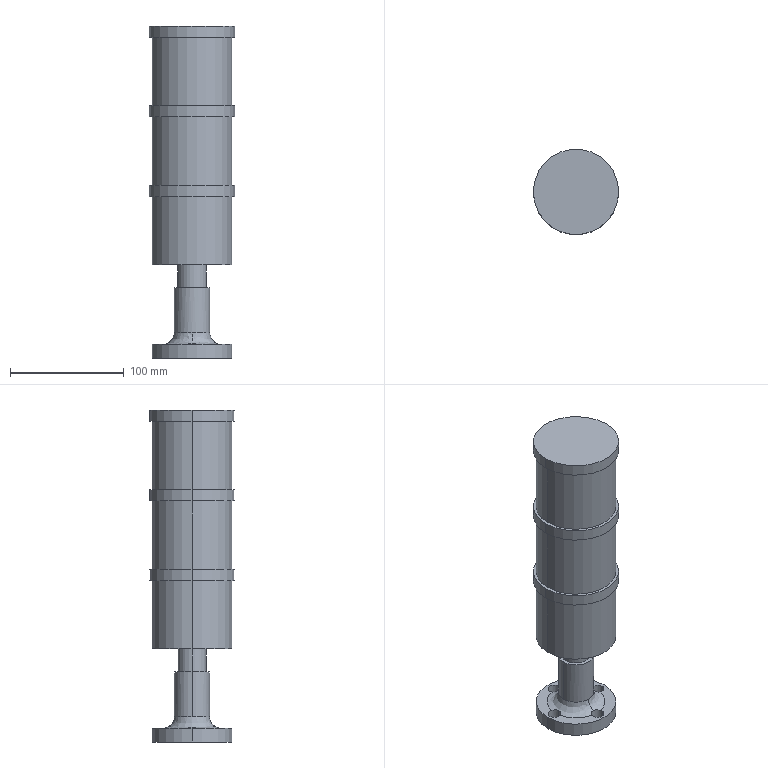Part | SolidWorks | features BaseBody 1 | 1 solid | 66 faces | box 75 x 75 x 292 mm | volume 894317 mm3 | cylinder 47 | plane 17 | spline 2 | commonest cylinder face diameters 5.5 x8 11 x8 70 x8 75 x6 14 x5 25 x4